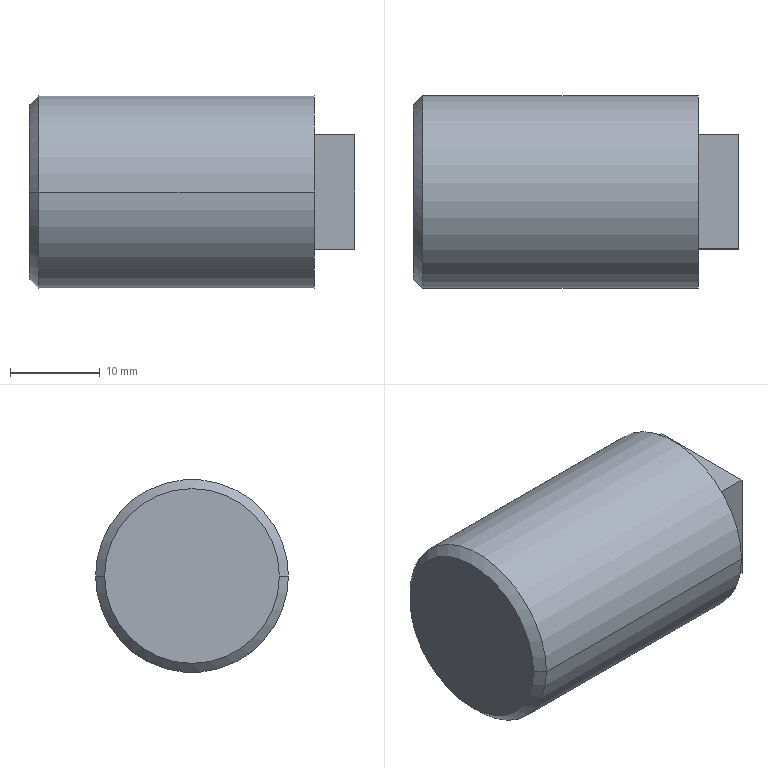Part | NX | features BREP 1 | 1 solid | 15 faces | box 36.22 x 21.488 x 21.488 mm | volume 11606 mm3 | plane 7 | cylinder 4 | cone 4 | commonest cylinder face diameters 7.938 x2 21.488 x2
STEP:
#1=CARTESIAN_POINT('',(0.,-10.744,0.));
#2=VERTEX_POINT('',#1);
#3=CARTESIAN_POINT('',(0.,10.744,0.));
#4=VERTEX_POINT('',#3);
#5=CARTESIAN_POINT('',(0.,0.,0.));
#6=DIRECTION('',(-1.,0.,0.));
#7=DIRECTION('',(0.,-1.,0.));
#8=AXIS2_PLACEMENT_3D('',#5,#6,#7);
#9=CIRCLE('',#8,10.744);
#10=EDGE_CURVE('',#2,#4,#9,.T.);
#11=ORIENTED_EDGE('',*,*,#10,.F.);
#12=CARTESIAN_POINT('',(0.,0.,0.));
#13=DIRECTION('',(-1.,0.,0.));
#14=DIRECTION('',(0.,1.,0.));
#15=AXIS2_PLACEMENT_3D('',#12,#13,#14);
#16=CIRCLE('',#15,10.744);
#17=EDGE_CURVE('',#4,#2,#16,.T.);
#18=ORIENTED_EDGE('',*,*,#17,.F.);
#19=EDGE_LOOP('',(#11,#18));
#20=FACE_BOUND('',#19,.T.);
#21=CARTESIAN_POINT('',(0.,6.35,-6.35));
#22=VERTEX_POINT('',#21);
#23=CARTESIAN_POINT('',(0.,6.35,6.35));
#24=VERTEX_POINT('',#23);
#25=CARTESIAN_POINT('',(0.,6.35,-6.35));
#26=DIRECTION('',(0.,0.,1.));
#27=VECTOR('',#26,1000.);
#28=LINE('',#25,#27);
#29=EDGE_CURVE('',#22,#24,#28,.T.);
#30=ORIENTED_EDGE('',*,*,#29,.F.);
#31=CARTESIAN_POINT('',(0.,-6.35,-6.35));
#32=VERTEX_POINT('',#31);
#33=CARTESIAN_POINT('',(0.,-6.35,-6.35));
#34=DIRECTION('',(0.,1.,0.));
#35=VECTOR('',#34,1000.);
#36=LINE('',#33,#35);
#37=EDGE_CURVE('',#32,#22,#36,.T.);
#38=ORIENTED_EDGE('',*,*,#37,.F.);
#39=CARTESIAN_POINT('',(0.,-6.35,6.35));
#40=VERTEX_POINT('',#39);
#41=CARTESIAN_POINT('',(0.,-6.35,6.35));
#42=DIRECTION('',(0.,0.,-1.));
#43=VECTOR('',#42,1000.);
#44=LINE('',#41,#43);
#45=EDGE_CURVE('',#40,#32,#44,.T.);
#46=ORIENTED_EDGE('',*,*,#45,.F.);
#47=CARTESIAN_POINT('',(0.,6.35,6.35));
#48=DIRECTION('',(0.,-1.,0.));
#49=VECTOR('',#48,1000.);
#50=LINE('',#47,#49);
#51=EDGE_CURVE('',#24,#40,#50,.T.);
#52=ORIENTED_EDGE('',*,*,#51,.F.);
#53=EDGE_LOOP('',(#30,#38,#46,#52));
#54=FACE_BOUND('',#53,.T.);
#55=CARTESIAN_POINT('',(0.,0.,0.));
#56=DIRECTION('',(-1.,0.,0.));
#57=DIRECTION('',(0.,0.,1.));
#58=AXIS2_PLACEMENT_3D('',#55,#56,#57);
#59=PLANE('',#58);
#60=ADVANCED_FACE('',(#20,#54),#59,.F.);
#61=CARTESIAN_POINT('',(-30.734,-10.744,0.));
#62=VERTEX_POINT('',#61);
#63=CARTESIAN_POINT('',(0.,-10.744,0.));
#64=DIRECTION('',(-1.,0.,0.));
#65=VECTOR('',#64,1000.);
#66=LINE('',#63,#65);
#67=EDGE_CURVE('',#2,#62,#66,.T.);
#68=ORIENTED_EDGE('',*,*,#67,.T.);
#69=CARTESIAN_POINT('',(-30.734,10.744,0.));
#70=VERTEX_POINT('',#69);
#71=CARTESIAN_POINT('',(-30.734,0.,0.));
#72=DIRECTION('',(-1.,0.,0.));
#73=DIRECTION('',(0.,1.,0.));
#74=AXIS2_PLACEMENT_3D('',#71,#72,#73);
#75=CIRCLE('',#74,10.744);
#76=EDGE_CURVE('',#70,#62,#75,.T.);
#77=ORIENTED_EDGE('',*,*,#76,.F.);
#78=CARTESIAN_POINT('',(0.,10.744,0.));
#79=DIRECTION('',(-1.,0.,0.));
#80=VECTOR('',#79,1000.);
#81=LINE('',#78,#80);
#82=EDGE_CURVE('',#4,#70,#81,.T.);
#83=ORIENTED_EDGE('',*,*,#82,.F.);
#84=ORIENTED_EDGE('',*,*,#17,.T.);
#85=EDGE_LOOP('',(#68,#77,#83,#84));
#86=FACE_BOUND('',#85,.T.);
#87=CARTESIAN_POINT('',(0.,0.,0.));
#88=DIRECTION('',(-1.,0.,0.));
#89=DIRECTION('',(0.,1.,0.));
#90=AXIS2_PLACEMENT_3D('',#87,#88,#89);
#91=CYLINDRICAL_SURFACE('',#90,10.744);
#92=ADVANCED_FACE('',(#86),#91,.T.);
#93=ORIENTED_EDGE('',*,*,#82,.T.);
#94=CARTESIAN_POINT('',(-30.734,0.,0.));
#95=DIRECTION('',(-1.,0.,0.));
#96=DIRECTION('',(0.,-1.,0.));
#97=AXIS2_PLACEMENT_3D('',#94,#95,#96);
#98=CIRCLE('',#97,10.744);
#99=EDGE_CURVE('',#62,#70,#98,.T.);
#100=ORIENTED_EDGE('',*,*,#99,.F.);
#101=ORIENTED_EDGE('',*,*,#67,.F.);
#102=ORIENTED_EDGE('',*,*,#10,.T.);
#103=EDGE_LOOP('',(#93,#100,#101,#102));
#104=FACE_BOUND('',#103,.T.);
#105=CARTESIAN_POINT('',(0.,0.,0.));
#106=DIRECTION('',(-1.,0.,0.));
#107=DIRECTION('',(0.,1.,0.));
#108=AXIS2_PLACEMENT_3D('',#105,#106,#107);
#109=CYLINDRICAL_SURFACE('',#108,10.744);
#110=ADVANCED_FACE('',(#104),#109,.T.);
#111=CARTESIAN_POINT('',(-31.75,-9.728,0.));
#112=VERTEX_POINT('',#111);
#113=CARTESIAN_POINT('',(-31.75,-9.728,0.));
#114=DIRECTION('',(0.7071,-0.7071,0.));
#115=VECTOR('',#114,1000.);
#116=LINE('',#113,#115);
#117=EDGE_CURVE('',#112,#62,#116,.T.);
#118=ORIENTED_EDGE('',*,*,#117,.T.);
#119=ORIENTED_EDGE('',*,*,#99,.T.);
#120=CARTESIAN_POINT('',(-31.75,9.728,0.));
#121=VERTEX_POINT('',#120);
#122=CARTESIAN_POINT('',(-31.75,9.728,0.));
#123=DIRECTION('',(0.7071,0.7071,0.));
#124=VECTOR('',#123,1000.);
#125=LINE('',#122,#124);
#126=EDGE_CURVE('',#121,#70,#125,.T.);
#127=ORIENTED_EDGE('',*,*,#126,.F.);
#128=CARTESIAN_POINT('',(-31.75,0.,0.));
#129=DIRECTION('',(-1.,0.,0.));
#130=DIRECTION('',(0.,-1.,0.));
#131=AXIS2_PLACEMENT_3D('',#128,#129,#130);
#132=CIRCLE('',#131,9.728);
#133=EDGE_CURVE('',#112,#121,#132,.T.);
#134=ORIENTED_EDGE('',*,*,#133,.F.);
#135=EDGE_LOOP('',(#118,#119,#127,#134));
#136=FACE_BOUND('',#135,.T.);
#137=CARTESIAN_POINT('',(-31.242,0.,0.));
#138=DIRECTION('',(1.,0.,0.));
#139=DIRECTION('',(0.,-1.,0.));
#140=AXIS2_PLACEMENT_3D('',#137,#138,#139);
#141=CONICAL_SURFACE('',#140,10.236,0.7854);
#142=ADVANCED_FACE('',(#136),#141,.T.);
#143=ORIENTED_EDGE('',*,*,#133,.T.);
#144=CARTESIAN_POINT('',(-31.75,0.,0.));
#145=DIRECTION('',(-1.,0.,0.));
#146=DIRECTION('',(0.,1.,0.));
#147=AXIS2_PLACEMENT_3D('',#144,#145,#146);
#148=CIRCLE('',#147,9.728);
#149=EDGE_CURVE('',#121,#112,#148,.T.);
#150=ORIENTED_EDGE('',*,*,#149,.T.);
#151=EDGE_LOOP('',(#143,#150));
#152=FACE_BOUND('',#151,.T.);
#153=CARTESIAN_POINT('',(-31.75,0.,0.));
#154=DIRECTION('',(-1.,0.,0.));
#155=DIRECTION('',(0.,0.,1.));
#156=AXIS2_PLACEMENT_3D('',#153,#154,#155);
#157=PLANE('',#156);
#158=ADVANCED_FACE('',(#152),#157,.T.);
#159=ORIENTED_EDGE('',*,*,#126,.T.);
#160=ORIENTED_EDGE('',*,*,#76,.T.);
#161=ORIENTED_EDGE('',*,*,#117,.F.);
#162=ORIENTED_EDGE('',*,*,#149,.F.);
#163=EDGE_LOOP('',(#159,#160,#161,#162));
#164=FACE_BOUND('',#163,.T.);
#165=CARTESIAN_POINT('',(-31.242,0.,0.));
#166=DIRECTION('',(1.,0.,0.));
#167=DIRECTION('',(0.,-1.,0.));
#168=AXIS2_PLACEMENT_3D('',#165,#166,#167);
#169=CONICAL_SURFACE('',#168,10.236,0.7854);
#170=ADVANCED_FACE('',(#164),#169,.T.);
#171=CARTESIAN_POINT('',(4.47,-6.35,6.35));
#172=VERTEX_POINT('',#171);
#173=CARTESIAN_POINT('',(0.,-6.35,6.35));
#174=DIRECTION('',(1.,0.,0.));
#175=VECTOR('',#174,1000.);
#176=LINE('',#173,#175);
#177=EDGE_CURVE('',#40,#172,#176,.T.);
#178=ORIENTED_EDGE('',*,*,#177,.T.);
#179=CARTESIAN_POINT('',(4.47,6.35,6.35));
#180=VERTEX_POINT('',#179);
#181=CARTESIAN_POINT('',(4.47,6.35,6.35));
#182=DIRECTION('',(0.,-1.,0.));
#183=VECTOR('',#182,1000.);
#184=LINE('',#181,#183);
#185=EDGE_CURVE('',#180,#172,#184,.T.);
#186=ORIENTED_EDGE('',*,*,#185,.F.);
#187=CARTESIAN_POINT('',(0.,6.35,6.35));
#188=DIRECTION('',(1.,0.,0.));
#189=VECTOR('',#188,1000.);
#190=LINE('',#187,#189);
#191=EDGE_CURVE('',#24,#180,#190,.T.);
#192=ORIENTED_EDGE('',*,*,#191,.F.);
#193=ORIENTED_EDGE('',*,*,#51,.T.);
#194=EDGE_LOOP('',(#178,#186,#192,#193));
#195=FACE_BOUND('',#194,.T.);
#196=CARTESIAN_POINT('',(0.,6.35,6.35));
#197=DIRECTION('',(0.,0.,1.));
#198=DIRECTION('',(1.,0.,0.));
#199=AXIS2_PLACEMENT_3D('',#196,#197,#198);
#200=PLANE('',#199);
#201=ADVANCED_FACE('',(#195),#200,.T.);
#202=ORIENTED_EDGE('',*,*,#191,.T.);
#203=CARTESIAN_POINT('',(4.47,6.35,-6.35));
#204=VERTEX_POINT('',#203);
#205=CARTESIAN_POINT('',(4.47,6.35,-6.35));
#206=DIRECTION('',(0.,0.,1.));
#207=VECTOR('',#206,1000.);
#208=LINE('',#205,#207);
#209=EDGE_CURVE('',#204,#180,#208,.T.);
#210=ORIENTED_EDGE('',*,*,#209,.F.);
#211=CARTESIAN_POINT('',(0.,6.35,-6.35));
#212=DIRECTION('',(1.,0.,0.));
#213=VECTOR('',#212,1000.);
#214=LINE('',#211,#213);
#215=EDGE_CURVE('',#22,#204,#214,.T.);
#216=ORIENTED_EDGE('',*,*,#215,.F.);
#217=ORIENTED_EDGE('',*,*,#29,.T.);
#218=EDGE_LOOP('',(#202,#210,#216,#217));
#219=FACE_BOUND('',#218,.T.);
#220=CARTESIAN_POINT('',(0.,6.35,-6.35));
#221=DIRECTION('',(0.,1.,0.));
#222=DIRECTION('',(1.,0.,0.));
#223=AXIS2_PLACEMENT_3D('',#220,#221,#222);
#224=PLANE('',#223);
#225=ADVANCED_FACE('',(#219),#224,.T.);
#226=ORIENTED_EDGE('',*,*,#215,.T.);
#227=CARTESIAN_POINT('',(4.47,-6.35,-6.35));
#228=VERTEX_POINT('',#227);
#229=CARTESIAN_POINT('',(4.47,-6.35,-6.35));
#230=DIRECTION('',(0.,1.,0.));
#231=VECTOR('',#230,1000.);
#232=LINE('',#229,#231);
#233=EDGE_CURVE('',#228,#204,#232,.T.);
#234=ORIENTED_EDGE('',*,*,#233,.F.);
#235=CARTESIAN_POINT('',(0.,-6.35,-6.35));
#236=DIRECTION('',(1.,0.,0.));
#237=VECTOR('',#236,1000.);
#238=LINE('',#235,#237);
#239=EDGE_CURVE('',#32,#228,#238,.T.);
#240=ORIENTED_EDGE('',*,*,#239,.F.);
#241=ORIENTED_EDGE('',*,*,#37,.T.);
#242=EDGE_LOOP('',(#226,#234,#240,#241));
#243=FACE_BOUND('',#242,.T.);
#244=CARTESIAN_POINT('',(0.,-6.35,-6.35));
#245=DIRECTION('',(0.,0.,-1.));
#246=DIRECTION('',(0.,-1.,0.));
#247=AXIS2_PLACEMENT_3D('',#244,#245,#246);
#248=PLANE('',#247);
#249=ADVANCED_FACE('',(#243),#248,.T.);
#250=ORIENTED_EDGE('',*,*,#239,.T.);
#251=CARTESIAN_POINT('',(4.47,-6.35,6.35));
#252=DIRECTION('',(0.,0.,-1.));
#253=VECTOR('',#252,1000.);
#254=LINE('',#251,#253);
#255=EDGE_CURVE('',#172,#228,#254,.T.);
#256=ORIENTED_EDGE('',*,*,#255,.F.);
#257=ORIENTED_EDGE('',*,*,#177,.F.);
#258=ORIENTED_EDGE('',*,*,#45,.T.);
#259=EDGE_LOOP('',(#250,#256,#257,#258));
#260=FACE_BOUND('',#259,.T.);
#261=CARTESIAN_POINT('',(0.,-6.35,6.35));
#262=DIRECTION('',(0.,-1.,0.));
#263=DIRECTION('',(0.,0.,-1.));
#264=AXIS2_PLACEMENT_3D('',#261,#262,#263);
#265=PLANE('',#264);
#266=ADVANCED_FACE('',(#260),#265,.T.);
#267=ORIENTED_EDGE('',*,*,#255,.T.);
#268=ORIENTED_EDGE('',*,*,#233,.T.);
#269=ORIENTED_EDGE('',*,*,#209,.T.);
#270=ORIENTED_EDGE('',*,*,#185,.T.);
#271=EDGE_LOOP('',(#267,#268,#269,#270));
#272=FACE_BOUND('',#271,.T.);
#273=CARTESIAN_POINT('',(4.47,3.969,0.));
#274=VERTEX_POINT('',#273);
#275=CARTESIAN_POINT('',(4.47,-3.969,0.));
#276=VERTEX_POINT('',#275);
#277=CARTESIAN_POINT('',(4.47,0.,0.));
#278=DIRECTION('',(1.,0.,0.));
#279=DIRECTION('',(0.,1.,0.));
#280=AXIS2_PLACEMENT_3D('',#277,#278,#279);
#281=CIRCLE('',#280,3.969);
#282=EDGE_CURVE('',#274,#276,#281,.T.);
#283=ORIENTED_EDGE('',*,*,#282,.F.);
#284=CARTESIAN_POINT('',(4.47,0.,0.));
#285=DIRECTION('',(1.,0.,0.));
#286=DIRECTION('',(0.,-1.,0.));
#287=AXIS2_PLACEMENT_3D('',#284,#285,#286);
#288=CIRCLE('',#287,3.969);
#289=EDGE_CURVE('',#276,#274,#288,.T.);
#290=ORIENTED_EDGE('',*,*,#289,.F.);
#291=EDGE_LOOP('',(#283,#290));
#292=FACE_BOUND('',#291,.T.);
#293=CARTESIAN_POINT('',(4.47,0.,0.));
#294=DIRECTION('',(1.,0.,0.));
#295=DIRECTION('',(0.,1.,0.));
#296=AXIS2_PLACEMENT_3D('',#293,#294,#295);
#297=PLANE('',#296);
#298=ADVANCED_FACE('',(#272,#292),#297,.T.);
#299=CARTESIAN_POINT('',(-6.108,3.969,0.));
#300=VERTEX_POINT('',#299);
#301=CARTESIAN_POINT('',(-6.108,3.969,0.));
#302=DIRECTION('',(1.,0.,0.));
#303=VECTOR('',#302,1000.);
#304=LINE('',#301,#303);
#305=EDGE_CURVE('',#274,#300,#304,.F.);
#306=ORIENTED_EDGE('',*,*,#305,.T.);
#307=CARTESIAN_POINT('',(-6.108,-3.969,0.));
#308=VERTEX_POINT('',#307);
#309=CARTESIAN_POINT('',(-6.108,0.,0.));
#310=DIRECTION('',(1.,0.,0.));
#311=DIRECTION('',(0.,-1.,0.));
#312=AXIS2_PLACEMENT_3D('',#309,#310,#311);
#313=CIRCLE('',#312,3.969);
#314=EDGE_CURVE('',#308,#300,#313,.T.);
#315=ORIENTED_EDGE('',*,*,#314,.F.);
#316=CARTESIAN_POINT('',(-6.108,-3.969,0.));
#317=DIRECTION('',(1.,0.,0.));
#318=VECTOR('',#317,1000.);
#319=LINE('',#316,#318);
#320=EDGE_CURVE('',#276,#308,#319,.F.);
#321=ORIENTED_EDGE('',*,*,#320,.F.);
#322=ORIENTED_EDGE('',*,*,#289,.T.);
#323=EDGE_LOOP('',(#306,#315,#321,#322));
#324=FACE_BOUND('',#323,.T.);
#325=CARTESIAN_POINT('',(-11.265,0.,0.));
#326=DIRECTION('',(1.,0.,0.));
#327=DIRECTION('',(0.,-1.,0.));
#328=AXIS2_PLACEMENT_3D('',#325,#326,#327);
#329=CYLINDRICAL_SURFACE('',#328,3.969);
#330=ADVANCED_FACE('',(#324),#329,.F.);
#331=ORIENTED_EDGE('',*,*,#320,.T.);
#332=CARTESIAN_POINT('',(-6.108,0.,0.));
#333=DIRECTION('',(-1.,0.,0.));
#334=DIRECTION('',(0.,-1.,0.));
#335=AXIS2_PLACEMENT_3D('',#332,#333,#334);
#336=CIRCLE('',#335,3.969);
#337=EDGE_CURVE('',#308,#300,#336,.T.);
#338=ORIENTED_EDGE('',*,*,#337,.T.);
#339=ORIENTED_EDGE('',*,*,#305,.F.);
#340=ORIENTED_EDGE('',*,*,#282,.T.);
#341=EDGE_LOOP('',(#331,#338,#339,#340));
#342=FACE_BOUND('',#341,.T.);
#343=CARTESIAN_POINT('',(-11.265,0.,0.));
#344=DIRECTION('',(1.,0.,0.));
#345=DIRECTION('',(0.,-1.,0.));
#346=AXIS2_PLACEMENT_3D('',#343,#344,#345);
#347=CYLINDRICAL_SURFACE('',#346,3.969);
#348=ADVANCED_FACE('',(#342),#347,.F.);
#349=CARTESIAN_POINT('',(-10.516,0.,0.));
#350=VERTEX_POINT('',#349);
#351=CARTESIAN_POINT('',(-10.516,0.,0.));
#352=DIRECTION('',(0.7431,0.6691,0.));
#353=VECTOR('',#352,1000.);
#354=LINE('',#351,#353);
#355=EDGE_CURVE('',#350,#300,#354,.T.);
#356=ORIENTED_EDGE('',*,*,#355,.T.);
#357=ORIENTED_EDGE('',*,*,#337,.F.);
#358=CARTESIAN_POINT('',(-10.516,0.,0.));
#359=DIRECTION('',(0.7431,-0.6691,0.));
#360=VECTOR('',#359,1000.);
#361=LINE('',#358,#360);
#362=EDGE_CURVE('',#350,#308,#361,.T.);
#363=ORIENTED_EDGE('',*,*,#362,.F.);
#364=EDGE_LOOP('',(#356,#357,#363));
#365=FACE_BOUND('',#364,.T.);
#366=CARTESIAN_POINT('',(-8.268,0.,0.));
#367=DIRECTION('',(1.,0.,0.));
#368=DIRECTION('',(0.,-1.,0.));
#369=AXIS2_PLACEMENT_3D('',#366,#367,#368);
#370=CONICAL_SURFACE('',#369,2.024,0.733);
#371=ADVANCED_FACE('',(#365),#370,.F.);
#372=ORIENTED_EDGE('',*,*,#314,.T.);
#373=ORIENTED_EDGE('',*,*,#355,.F.);
#374=ORIENTED_EDGE('',*,*,#362,.T.);
#375=EDGE_LOOP('',(#372,#373,#374));
#376=FACE_BOUND('',#375,.T.);
#377=CARTESIAN_POINT('',(-8.268,0.,0.));
#378=DIRECTION('',(1.,0.,0.));
#379=DIRECTION('',(0.,-1.,0.));
#380=AXIS2_PLACEMENT_3D('',#377,#378,#379);
#381=CONICAL_SURFACE('',#380,2.024,0.733);
#382=ADVANCED_FACE('',(#376),#381,.F.);
#383=CLOSED_SHELL('',(#60,#92,#110,#142,#158,#170,#201,#225,#249,#266,#298,#330,#348,#371,#382));
#384=MANIFOLD_SOLID_BREP('',#383);
#385=(LENGTH_UNIT()NAMED_UNIT(*)SI_UNIT(.MILLI.,.METRE.));
#386=UNCERTAINTY_MEASURE_WITH_UNIT(LENGTH_MEASURE(0.00001),#385,'','');
#387=(NAMED_UNIT(*)PLANE_ANGLE_UNIT()SI_UNIT($,.RADIAN.));
#388=(NAMED_UNIT(*)SI_UNIT($,.STERADIAN.)SOLID_ANGLE_UNIT());
#389=(GEOMETRIC_REPRESENTATION_CONTEXT(3)GLOBAL_UNCERTAINTY_ASSIGNED_CONTEXT((#386))GLOBAL_UNIT_ASSIGNED_CONTEXT((#385,#387,#388))REPRESENTATION_CONTEXT('',''));
#390=ADVANCED_BREP_SHAPE_REPRESENTATION('',(#384),#389);